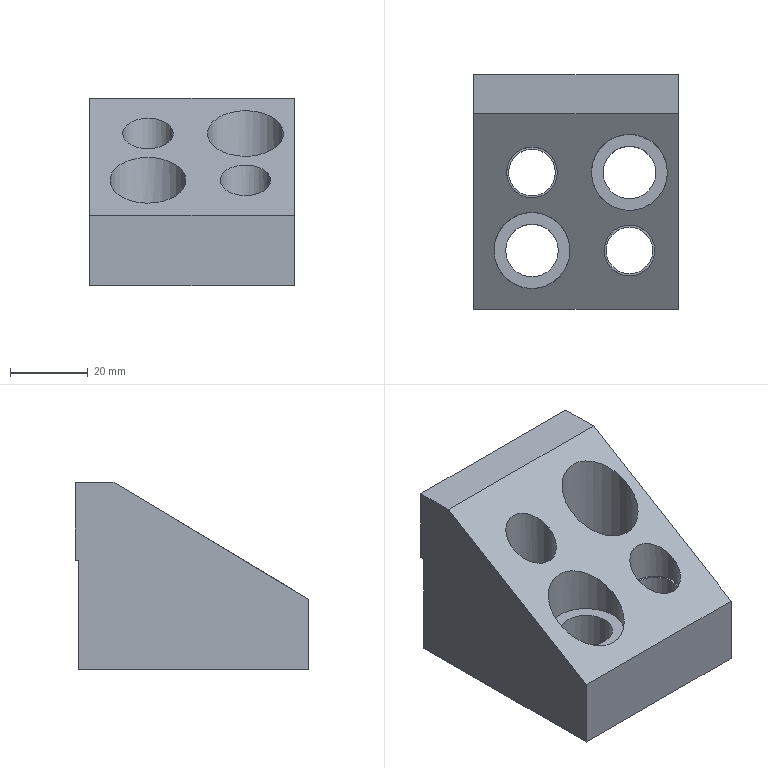Part | NX | features solid 2 | 1 solid | 21 faces | box 52.578 x 60 x 48 mm | volume 89054 mm3 | plane 13 | cylinder 8 | commonest cylinder face diameters 12 x2 13 x2 13.5 x2 19.5 x2
STEP:
#1=CARTESIAN_POINT('',(-464.,-150.,-55.));
#2=VERTEX_POINT('',#1);
#3=CARTESIAN_POINT('',(-470.,-150.,-55.));
#4=DIRECTION('',(0.,0.,1.));
#5=DIRECTION('',(1.,0.,0.));
#6=AXIS2_PLACEMENT_3D('',#3,#4,#5);
#7=CIRCLE('',#6,6.);
#8=EDGE_CURVE('',#2,#2,#7,.F.);
#9=ORIENTED_EDGE('',*,*,#8,.F.);
#10=EDGE_LOOP('',(#9));
#11=FACE_BOUND('',#10,.T.);
#12=CARTESIAN_POINT('',(-489.,-130.,-55.));
#13=VERTEX_POINT('',#12);
#14=CARTESIAN_POINT('',(-495.,-130.,-55.));
#15=DIRECTION('',(0.,0.,1.));
#16=DIRECTION('',(1.,0.,0.));
#17=AXIS2_PLACEMENT_3D('',#14,#15,#16);
#18=CIRCLE('',#17,6.);
#19=EDGE_CURVE('',#13,#13,#18,.F.);
#20=ORIENTED_EDGE('',*,*,#19,.F.);
#21=EDGE_LOOP('',(#20));
#22=FACE_BOUND('',#21,.T.);
#23=CARTESIAN_POINT('',(-488.25,-150.,-55.));
#24=VERTEX_POINT('',#23);
#25=CARTESIAN_POINT('',(-495.,-150.,-55.));
#26=DIRECTION('',(0.,0.,1.));
#27=DIRECTION('',(1.,0.,0.));
#28=AXIS2_PLACEMENT_3D('',#25,#26,#27);
#29=CIRCLE('',#28,6.75);
#30=EDGE_CURVE('',#24,#24,#29,.F.);
#31=ORIENTED_EDGE('',*,*,#30,.F.);
#32=EDGE_LOOP('',(#31));
#33=FACE_BOUND('',#32,.T.);
#34=CARTESIAN_POINT('',(-463.25,-130.,-55.));
#35=VERTEX_POINT('',#34);
#36=CARTESIAN_POINT('',(-470.,-130.,-55.));
#37=DIRECTION('',(0.,0.,1.));
#38=DIRECTION('',(1.,0.,0.));
#39=AXIS2_PLACEMENT_3D('',#36,#37,#38);
#40=CIRCLE('',#39,6.75);
#41=EDGE_CURVE('',#35,#35,#40,.F.);
#42=ORIENTED_EDGE('',*,*,#41,.F.);
#43=EDGE_LOOP('',(#42));
#44=FACE_BOUND('',#43,.T.);
#45=CARTESIAN_POINT('',(-510.,-106.,-55.));
#46=VERTEX_POINT('',#45);
#47=CARTESIAN_POINT('',(-510.,-165.,-55.));
#48=VERTEX_POINT('',#47);
#49=CARTESIAN_POINT('',(-510.,35.09,-55.));
#50=DIRECTION('',(0.,1.,0.));
#51=VECTOR('',#50,1000.);
#52=LINE('',#49,#51);
#53=EDGE_CURVE('',#46,#48,#52,.F.);
#54=ORIENTED_EDGE('',*,*,#53,.F.);
#55=CARTESIAN_POINT('',(-457.422,-106.,-55.));
#56=VERTEX_POINT('',#55);
#57=CARTESIAN_POINT('',(-457.422,-106.,-55.));
#58=DIRECTION('',(1.,0.,0.));
#59=VECTOR('',#58,1000.);
#60=LINE('',#57,#59);
#61=EDGE_CURVE('',#56,#46,#60,.F.);
#62=ORIENTED_EDGE('',*,*,#61,.F.);
#63=CARTESIAN_POINT('',(-457.422,-165.,-55.));
#64=VERTEX_POINT('',#63);
#65=CARTESIAN_POINT('',(-457.422,35.09,-55.));
#66=DIRECTION('',(0.,-1.,0.));
#67=VECTOR('',#66,1000.);
#68=LINE('',#65,#67);
#69=EDGE_CURVE('',#56,#64,#68,.T.);
#70=ORIENTED_EDGE('',*,*,#69,.T.);
#71=CARTESIAN_POINT('',(-415.478,-165.,-55.));
#72=DIRECTION('',(1.,0.,0.));
#73=VECTOR('',#72,1000.);
#74=LINE('',#71,#73);
#75=EDGE_CURVE('',#64,#48,#74,.F.);
#76=ORIENTED_EDGE('',*,*,#75,.T.);
#77=EDGE_LOOP('',(#54,#62,#70,#76));
#78=FACE_BOUND('',#77,.T.);
#79=CARTESIAN_POINT('',(-415.478,35.09,-55.));
#80=DIRECTION('',(0.,0.,1.));
#81=DIRECTION('',(1.,0.,0.));
#82=AXIS2_PLACEMENT_3D('',#79,#80,#81);
#83=PLANE('',#82);
#84=ADVANCED_FACE('',(#11,#22,#33,#44,#78),#83,.F.);
#85=CARTESIAN_POINT('',(-510.,-115.,-7.));
#86=VERTEX_POINT('',#85);
#87=CARTESIAN_POINT('',(-510.,-105.,-7.));
#88=VERTEX_POINT('',#87);
#89=CARTESIAN_POINT('',(-510.,-105.,-7.));
#90=DIRECTION('',(0.,-1.,0.));
#91=VECTOR('',#90,1000.);
#92=LINE('',#89,#91);
#93=EDGE_CURVE('',#86,#88,#92,.F.);
#94=ORIENTED_EDGE('',*,*,#93,.F.);
#95=CARTESIAN_POINT('',(-457.422,-115.,-7.));
#96=VERTEX_POINT('',#95);
#97=CARTESIAN_POINT('',(-457.422,-115.,-7.));
#98=DIRECTION('',(1.,0.,0.));
#99=VECTOR('',#98,1000.);
#100=LINE('',#97,#99);
#101=EDGE_CURVE('',#96,#86,#100,.F.);
#102=ORIENTED_EDGE('',*,*,#101,.F.);
#103=CARTESIAN_POINT('',(-457.422,-105.,-7.));
#104=VERTEX_POINT('',#103);
#105=CARTESIAN_POINT('',(-457.422,-105.,-7.));
#106=DIRECTION('',(0.,-1.,0.));
#107=VECTOR('',#106,1000.);
#108=LINE('',#105,#107);
#109=EDGE_CURVE('',#104,#96,#108,.T.);
#110=ORIENTED_EDGE('',*,*,#109,.F.);
#111=CARTESIAN_POINT('',(-457.422,-105.,-7.));
#112=DIRECTION('',(-1.,0.,0.));
#113=VECTOR('',#112,1000.);
#114=LINE('',#111,#113);
#115=EDGE_CURVE('',#104,#88,#114,.T.);
#116=ORIENTED_EDGE('',*,*,#115,.T.);
#117=EDGE_LOOP('',(#94,#102,#110,#116));
#118=FACE_BOUND('',#117,.T.);
#119=CARTESIAN_POINT('',(-457.422,-105.,-7.));
#120=DIRECTION('',(0.,0.,-1.));
#121=DIRECTION('',(-1.,0.,0.));
#122=AXIS2_PLACEMENT_3D('',#119,#120,#121);
#123=PLANE('',#122);
#124=ADVANCED_FACE('',(#118),#123,.F.);
#125=CARTESIAN_POINT('',(-457.422,-105.,-27.));
#126=VERTEX_POINT('',#125);
#127=CARTESIAN_POINT('',(-457.422,-106.,-27.));
#128=VERTEX_POINT('',#127);
#129=CARTESIAN_POINT('',(-457.422,-105.,-27.));
#130=DIRECTION('',(0.,-1.,0.));
#131=VECTOR('',#130,1000.);
#132=LINE('',#129,#131);
#133=EDGE_CURVE('',#126,#128,#132,.T.);
#134=ORIENTED_EDGE('',*,*,#133,.F.);
#135=CARTESIAN_POINT('',(-457.422,-105.,-67.));
#136=DIRECTION('',(0.,0.,1.));
#137=VECTOR('',#136,1000.);
#138=LINE('',#135,#137);
#139=EDGE_CURVE('',#126,#104,#138,.T.);
#140=ORIENTED_EDGE('',*,*,#139,.T.);
#141=ORIENTED_EDGE('',*,*,#109,.T.);
#142=CARTESIAN_POINT('',(-457.422,-165.,-37.));
#143=VERTEX_POINT('',#142);
#144=CARTESIAN_POINT('',(-457.422,-134.118,-18.471));
#145=DIRECTION('',(0.,-0.8575,-0.5145));
#146=VECTOR('',#145,1000.);
#147=LINE('',#144,#146);
#148=EDGE_CURVE('',#143,#96,#147,.F.);
#149=ORIENTED_EDGE('',*,*,#148,.F.);
#150=CARTESIAN_POINT('',(-457.422,-165.,-67.));
#151=DIRECTION('',(0.,0.,1.));
#152=VECTOR('',#151,1000.);
#153=LINE('',#150,#152);
#154=EDGE_CURVE('',#64,#143,#153,.T.);
#155=ORIENTED_EDGE('',*,*,#154,.F.);
#156=ORIENTED_EDGE('',*,*,#69,.F.);
#157=CARTESIAN_POINT('',(-457.422,-106.,-27.));
#158=DIRECTION('',(0.,0.,-1.));
#159=VECTOR('',#158,1000.);
#160=LINE('',#157,#159);
#161=EDGE_CURVE('',#128,#56,#160,.T.);
#162=ORIENTED_EDGE('',*,*,#161,.F.);
#163=EDGE_LOOP('',(#134,#140,#141,#149,#155,#156,#162));
#164=FACE_BOUND('',#163,.T.);
#165=CARTESIAN_POINT('',(-457.422,-105.,-67.));
#166=DIRECTION('',(-1.,0.,0.));
#167=DIRECTION('',(0.,0.,1.));
#168=AXIS2_PLACEMENT_3D('',#165,#166,#167);
#169=PLANE('',#168);
#170=ADVANCED_FACE('',(#164),#169,.F.);
#171=CARTESIAN_POINT('',(-510.,-165.,-37.));
#172=VERTEX_POINT('',#171);
#173=CARTESIAN_POINT('',(-510.,-165.,-67.));
#174=DIRECTION('',(0.,0.,1.));
#175=VECTOR('',#174,1000.);
#176=LINE('',#173,#175);
#177=EDGE_CURVE('',#48,#172,#176,.T.);
#178=ORIENTED_EDGE('',*,*,#177,.F.);
#179=ORIENTED_EDGE('',*,*,#75,.F.);
#180=ORIENTED_EDGE('',*,*,#154,.T.);
#181=CARTESIAN_POINT('',(-457.422,-165.,-37.));
#182=DIRECTION('',(1.,0.,0.));
#183=VECTOR('',#182,1000.);
#184=LINE('',#181,#183);
#185=EDGE_CURVE('',#172,#143,#184,.T.);
#186=ORIENTED_EDGE('',*,*,#185,.F.);
#187=EDGE_LOOP('',(#178,#179,#180,#186));
#188=FACE_BOUND('',#187,.T.);
#189=CARTESIAN_POINT('',(-457.422,-165.,-67.));
#190=DIRECTION('',(0.,-1.,0.));
#191=DIRECTION('',(0.,0.,1.));
#192=AXIS2_PLACEMENT_3D('',#189,#190,#191);
#193=PLANE('',#192);
#194=ADVANCED_FACE('',(#188),#193,.T.);
#195=CARTESIAN_POINT('',(-510.,-105.,-27.));
#196=VERTEX_POINT('',#195);
#197=CARTESIAN_POINT('',(-457.422,-105.,-27.));
#198=DIRECTION('',(1.,0.,0.));
#199=VECTOR('',#198,1000.);
#200=LINE('',#197,#199);
#201=EDGE_CURVE('',#196,#126,#200,.T.);
#202=ORIENTED_EDGE('',*,*,#201,.F.);
#203=CARTESIAN_POINT('',(-510.,-105.,-67.));
#204=DIRECTION('',(0.,0.,1.));
#205=VECTOR('',#204,1000.);
#206=LINE('',#203,#205);
#207=EDGE_CURVE('',#196,#88,#206,.T.);
#208=ORIENTED_EDGE('',*,*,#207,.T.);
#209=ORIENTED_EDGE('',*,*,#115,.F.);
#210=ORIENTED_EDGE('',*,*,#139,.F.);
#211=EDGE_LOOP('',(#202,#208,#209,#210));
#212=FACE_BOUND('',#211,.T.);
#213=CARTESIAN_POINT('',(-457.422,-105.,-67.));
#214=DIRECTION('',(0.,-1.,0.));
#215=DIRECTION('',(0.,0.,1.));
#216=AXIS2_PLACEMENT_3D('',#213,#214,#215);
#217=PLANE('',#216);
#218=ADVANCED_FACE('',(#212),#217,.F.);
#219=CARTESIAN_POINT('',(-470.,-143.5,-24.1));
#220=VERTEX_POINT('',#219);
#221=CARTESIAN_POINT('',(-470.,-150.,-28.));
#222=DIRECTION('',(0.,-0.5145,0.8575));
#223=DIRECTION('',(0.,0.8575,0.5145));
#224=AXIS2_PLACEMENT_3D('',#221,#222,#223);
#225=ELLIPSE('',#224,7.58,6.5);
#226=EDGE_CURVE('',#220,#220,#225,.T.);
#227=ORIENTED_EDGE('',*,*,#226,.F.);
#228=EDGE_LOOP('',(#227));
#229=FACE_BOUND('',#228,.T.);
#230=CARTESIAN_POINT('',(-495.,-123.5,-12.1));
#231=VERTEX_POINT('',#230);
#232=CARTESIAN_POINT('',(-495.,-130.,-16.));
#233=DIRECTION('',(0.,-0.5145,0.8575));
#234=DIRECTION('',(0.,0.8575,0.5145));
#235=AXIS2_PLACEMENT_3D('',#232,#233,#234);
#236=ELLIPSE('',#235,7.58,6.5);
#237=EDGE_CURVE('',#231,#231,#236,.T.);
#238=ORIENTED_EDGE('',*,*,#237,.F.);
#239=EDGE_LOOP('',(#238));
#240=FACE_BOUND('',#239,.T.);
#241=CARTESIAN_POINT('',(-495.,-140.25,-22.15));
#242=VERTEX_POINT('',#241);
#243=CARTESIAN_POINT('',(-495.,-150.,-28.));
#244=DIRECTION('',(0.,-0.5145,0.8575));
#245=DIRECTION('',(0.,0.8575,0.5145));
#246=AXIS2_PLACEMENT_3D('',#243,#244,#245);
#247=ELLIPSE('',#246,11.37,9.75);
#248=EDGE_CURVE('',#242,#242,#247,.T.);
#249=ORIENTED_EDGE('',*,*,#248,.F.);
#250=EDGE_LOOP('',(#249));
#251=FACE_BOUND('',#250,.T.);
#252=CARTESIAN_POINT('',(-470.,-120.25,-10.15));
#253=VERTEX_POINT('',#252);
#254=CARTESIAN_POINT('',(-470.,-130.,-16.));
#255=DIRECTION('',(0.,-0.5145,0.8575));
#256=DIRECTION('',(0.,0.8575,0.5145));
#257=AXIS2_PLACEMENT_3D('',#254,#255,#256);
#258=ELLIPSE('',#257,11.37,9.75);
#259=EDGE_CURVE('',#253,#253,#258,.T.);
#260=ORIENTED_EDGE('',*,*,#259,.F.);
#261=EDGE_LOOP('',(#260));
#262=FACE_BOUND('',#261,.T.);
#263=CARTESIAN_POINT('',(-510.,-115.,-7.));
#264=DIRECTION('',(0.,0.8575,0.5145));
#265=VECTOR('',#264,1000.);
#266=LINE('',#263,#265);
#267=EDGE_CURVE('',#172,#86,#266,.T.);
#268=ORIENTED_EDGE('',*,*,#267,.F.);
#269=ORIENTED_EDGE('',*,*,#185,.T.);
#270=ORIENTED_EDGE('',*,*,#148,.T.);
#271=ORIENTED_EDGE('',*,*,#101,.T.);
#272=EDGE_LOOP('',(#268,#269,#270,#271));
#273=FACE_BOUND('',#272,.T.);
#274=CARTESIAN_POINT('',(-478.376,-115.,-7.));
#275=DIRECTION('',(0.,-0.5145,0.8575));
#276=DIRECTION('',(0.,0.8575,0.5145));
#277=AXIS2_PLACEMENT_3D('',#274,#275,#276);
#278=PLANE('',#277);
#279=ADVANCED_FACE('',(#229,#240,#251,#262,#273),#278,.T.);
#280=CARTESIAN_POINT('',(-510.,-106.,-27.));
#281=VERTEX_POINT('',#280);
#282=CARTESIAN_POINT('',(-457.422,-106.,-27.));
#283=DIRECTION('',(1.,0.,0.));
#284=VECTOR('',#283,1000.);
#285=LINE('',#282,#284);
#286=EDGE_CURVE('',#128,#281,#285,.F.);
#287=ORIENTED_EDGE('',*,*,#286,.T.);
#288=CARTESIAN_POINT('',(-510.,-105.,-27.));
#289=DIRECTION('',(0.,1.,0.));
#290=VECTOR('',#289,1000.);
#291=LINE('',#288,#290);
#292=EDGE_CURVE('',#281,#196,#291,.T.);
#293=ORIENTED_EDGE('',*,*,#292,.T.);
#294=ORIENTED_EDGE('',*,*,#201,.T.);
#295=ORIENTED_EDGE('',*,*,#133,.T.);
#296=EDGE_LOOP('',(#287,#293,#294,#295));
#297=FACE_BOUND('',#296,.T.);
#298=CARTESIAN_POINT('',(-457.422,-105.,-27.));
#299=DIRECTION('',(0.,0.,1.));
#300=DIRECTION('',(-1.,0.,0.));
#301=AXIS2_PLACEMENT_3D('',#298,#299,#300);
#302=PLANE('',#301);
#303=ADVANCED_FACE('',(#297),#302,.F.);
#304=CARTESIAN_POINT('',(-510.,-106.,-27.));
#305=DIRECTION('',(0.,0.,-1.));
#306=VECTOR('',#305,1000.);
#307=LINE('',#304,#306);
#308=EDGE_CURVE('',#281,#46,#307,.T.);
#309=ORIENTED_EDGE('',*,*,#308,.F.);
#310=ORIENTED_EDGE('',*,*,#286,.F.);
#311=ORIENTED_EDGE('',*,*,#161,.T.);
#312=ORIENTED_EDGE('',*,*,#61,.T.);
#313=EDGE_LOOP('',(#309,#310,#311,#312));
#314=FACE_BOUND('',#313,.T.);
#315=CARTESIAN_POINT('',(-457.422,-106.,-27.));
#316=DIRECTION('',(0.,1.,0.));
#317=DIRECTION('',(0.,0.,-1.));
#318=AXIS2_PLACEMENT_3D('',#315,#316,#317);
#319=PLANE('',#318);
#320=ADVANCED_FACE('',(#314),#319,.T.);
#321=ORIENTED_EDGE('',*,*,#53,.T.);
#322=ORIENTED_EDGE('',*,*,#177,.T.);
#323=ORIENTED_EDGE('',*,*,#267,.T.);
#324=ORIENTED_EDGE('',*,*,#93,.T.);
#325=ORIENTED_EDGE('',*,*,#207,.F.);
#326=ORIENTED_EDGE('',*,*,#292,.F.);
#327=ORIENTED_EDGE('',*,*,#308,.T.);
#328=EDGE_LOOP('',(#321,#322,#323,#324,#325,#326,#327));
#329=FACE_BOUND('',#328,.T.);
#330=CARTESIAN_POINT('',(-510.,0.,-7.));
#331=DIRECTION('',(1.,0.,0.));
#332=DIRECTION('',(0.,0.,-1.));
#333=AXIS2_PLACEMENT_3D('',#330,#331,#332);
#334=PLANE('',#333);
#335=ADVANCED_FACE('',(#329),#334,.F.);
#336=ORIENTED_EDGE('',*,*,#41,.T.);
#337=EDGE_LOOP('',(#336));
#338=FACE_BOUND('',#337,.T.);
#339=CARTESIAN_POINT('',(-476.75,-130.,-35.));
#340=VERTEX_POINT('',#339);
#341=CARTESIAN_POINT('',(-470.,-130.,-35.));
#342=DIRECTION('',(0.,0.,-1.));
#343=DIRECTION('',(-1.,0.,0.));
#344=AXIS2_PLACEMENT_3D('',#341,#342,#343);
#345=CIRCLE('',#344,6.75);
#346=EDGE_CURVE('',#340,#340,#345,.F.);
#347=ORIENTED_EDGE('',*,*,#346,.T.);
#348=EDGE_LOOP('',(#347));
#349=FACE_BOUND('',#348,.T.);
#350=CARTESIAN_POINT('',(-470.,-130.,-75.));
#351=DIRECTION('',(0.,0.,1.));
#352=DIRECTION('',(1.,0.,0.));
#353=AXIS2_PLACEMENT_3D('',#350,#351,#352);
#354=CYLINDRICAL_SURFACE('',#353,6.75);
#355=ADVANCED_FACE('',(#338,#349),#354,.F.);
#356=ORIENTED_EDGE('',*,*,#346,.F.);
#357=EDGE_LOOP('',(#356));
#358=FACE_BOUND('',#357,.T.);
#359=CARTESIAN_POINT('',(-460.25,-130.,-35.));
#360=VERTEX_POINT('',#359);
#361=CARTESIAN_POINT('',(-470.,-130.,-35.));
#362=DIRECTION('',(0.,0.,1.));
#363=DIRECTION('',(1.,0.,0.));
#364=AXIS2_PLACEMENT_3D('',#361,#362,#363);
#365=CIRCLE('',#364,9.75);
#366=EDGE_CURVE('',#360,#360,#365,.T.);
#367=ORIENTED_EDGE('',*,*,#366,.T.);
#368=EDGE_LOOP('',(#367));
#369=FACE_BOUND('',#368,.T.);
#370=CARTESIAN_POINT('',(-470.,-130.,-35.));
#371=DIRECTION('',(0.,0.,-1.));
#372=DIRECTION('',(-1.,0.,0.));
#373=AXIS2_PLACEMENT_3D('',#370,#371,#372);
#374=PLANE('',#373);
#375=ADVANCED_FACE('',(#358,#369),#374,.F.);
#376=ORIENTED_EDGE('',*,*,#259,.T.);
#377=EDGE_LOOP('',(#376));
#378=FACE_BOUND('',#377,.T.);
#379=ORIENTED_EDGE('',*,*,#366,.F.);
#380=EDGE_LOOP('',(#379));
#381=FACE_BOUND('',#380,.T.);
#382=CARTESIAN_POINT('',(-470.,-130.,-35.));
#383=DIRECTION('',(0.,0.,1.));
#384=DIRECTION('',(1.,0.,0.));
#385=AXIS2_PLACEMENT_3D('',#382,#383,#384);
#386=CYLINDRICAL_SURFACE('',#385,9.75);
#387=ADVANCED_FACE('',(#378,#381),#386,.F.);
#388=ORIENTED_EDGE('',*,*,#30,.T.);
#389=EDGE_LOOP('',(#388));
#390=FACE_BOUND('',#389,.T.);
#391=CARTESIAN_POINT('',(-501.75,-150.,-35.));
#392=VERTEX_POINT('',#391);
#393=CARTESIAN_POINT('',(-495.,-150.,-35.));
#394=DIRECTION('',(0.,0.,-1.));
#395=DIRECTION('',(-1.,0.,0.));
#396=AXIS2_PLACEMENT_3D('',#393,#394,#395);
#397=CIRCLE('',#396,6.75);
#398=EDGE_CURVE('',#392,#392,#397,.F.);
#399=ORIENTED_EDGE('',*,*,#398,.T.);
#400=EDGE_LOOP('',(#399));
#401=FACE_BOUND('',#400,.T.);
#402=CARTESIAN_POINT('',(-495.,-150.,-75.));
#403=DIRECTION('',(0.,0.,1.));
#404=DIRECTION('',(1.,0.,0.));
#405=AXIS2_PLACEMENT_3D('',#402,#403,#404);
#406=CYLINDRICAL_SURFACE('',#405,6.75);
#407=ADVANCED_FACE('',(#390,#401),#406,.F.);
#408=ORIENTED_EDGE('',*,*,#398,.F.);
#409=EDGE_LOOP('',(#408));
#410=FACE_BOUND('',#409,.T.);
#411=CARTESIAN_POINT('',(-485.25,-150.,-35.));
#412=VERTEX_POINT('',#411);
#413=CARTESIAN_POINT('',(-495.,-150.,-35.));
#414=DIRECTION('',(0.,0.,1.));
#415=DIRECTION('',(1.,0.,0.));
#416=AXIS2_PLACEMENT_3D('',#413,#414,#415);
#417=CIRCLE('',#416,9.75);
#418=EDGE_CURVE('',#412,#412,#417,.T.);
#419=ORIENTED_EDGE('',*,*,#418,.T.);
#420=EDGE_LOOP('',(#419));
#421=FACE_BOUND('',#420,.T.);
#422=CARTESIAN_POINT('',(-495.,-150.,-35.));
#423=DIRECTION('',(0.,0.,-1.));
#424=DIRECTION('',(-1.,0.,0.));
#425=AXIS2_PLACEMENT_3D('',#422,#423,#424);
#426=PLANE('',#425);
#427=ADVANCED_FACE('',(#410,#421),#426,.F.);
#428=ORIENTED_EDGE('',*,*,#248,.T.);
#429=EDGE_LOOP('',(#428));
#430=FACE_BOUND('',#429,.T.);
#431=ORIENTED_EDGE('',*,*,#418,.F.);
#432=EDGE_LOOP('',(#431));
#433=FACE_BOUND('',#432,.T.);
#434=CARTESIAN_POINT('',(-495.,-150.,-35.));
#435=DIRECTION('',(0.,0.,1.));
#436=DIRECTION('',(1.,0.,0.));
#437=AXIS2_PLACEMENT_3D('',#434,#435,#436);
#438=CYLINDRICAL_SURFACE('',#437,9.75);
#439=ADVANCED_FACE('',(#430,#433),#438,.F.);
#440=ORIENTED_EDGE('',*,*,#19,.T.);
#441=EDGE_LOOP('',(#440));
#442=FACE_BOUND('',#441,.T.);
#443=CARTESIAN_POINT('',(-501.,-130.,-35.));
#444=VERTEX_POINT('',#443);
#445=CARTESIAN_POINT('',(-495.,-130.,-35.));
#446=DIRECTION('',(0.,0.,-1.));
#447=DIRECTION('',(-1.,0.,0.));
#448=AXIS2_PLACEMENT_3D('',#445,#446,#447);
#449=CIRCLE('',#448,6.);
#450=EDGE_CURVE('',#444,#444,#449,.F.);
#451=ORIENTED_EDGE('',*,*,#450,.T.);
#452=EDGE_LOOP('',(#451));
#453=FACE_BOUND('',#452,.T.);
#454=CARTESIAN_POINT('',(-495.,-130.,-75.));
#455=DIRECTION('',(0.,0.,1.));
#456=DIRECTION('',(1.,0.,0.));
#457=AXIS2_PLACEMENT_3D('',#454,#455,#456);
#458=CYLINDRICAL_SURFACE('',#457,6.);
#459=ADVANCED_FACE('',(#442,#453),#458,.F.);
#460=ORIENTED_EDGE('',*,*,#450,.F.);
#461=EDGE_LOOP('',(#460));
#462=FACE_BOUND('',#461,.T.);
#463=CARTESIAN_POINT('',(-488.5,-130.,-35.));
#464=VERTEX_POINT('',#463);
#465=CARTESIAN_POINT('',(-495.,-130.,-35.));
#466=DIRECTION('',(0.,0.,1.));
#467=DIRECTION('',(1.,0.,0.));
#468=AXIS2_PLACEMENT_3D('',#465,#466,#467);
#469=CIRCLE('',#468,6.5);
#470=EDGE_CURVE('',#464,#464,#469,.T.);
#471=ORIENTED_EDGE('',*,*,#470,.T.);
#472=EDGE_LOOP('',(#471));
#473=FACE_BOUND('',#472,.T.);
#474=CARTESIAN_POINT('',(-495.,-130.,-35.));
#475=DIRECTION('',(0.,0.,-1.));
#476=DIRECTION('',(-1.,0.,0.));
#477=AXIS2_PLACEMENT_3D('',#474,#475,#476);
#478=PLANE('',#477);
#479=ADVANCED_FACE('',(#462,#473),#478,.F.);
#480=ORIENTED_EDGE('',*,*,#237,.T.);
#481=EDGE_LOOP('',(#480));
#482=FACE_BOUND('',#481,.T.);
#483=ORIENTED_EDGE('',*,*,#470,.F.);
#484=EDGE_LOOP('',(#483));
#485=FACE_BOUND('',#484,.T.);
#486=CARTESIAN_POINT('',(-495.,-130.,-35.));
#487=DIRECTION('',(0.,0.,1.));
#488=DIRECTION('',(1.,0.,0.));
#489=AXIS2_PLACEMENT_3D('',#486,#487,#488);
#490=CYLINDRICAL_SURFACE('',#489,6.5);
#491=ADVANCED_FACE('',(#482,#485),#490,.F.);
#492=ORIENTED_EDGE('',*,*,#8,.T.);
#493=EDGE_LOOP('',(#492));
#494=FACE_BOUND('',#493,.T.);
#495=CARTESIAN_POINT('',(-476.,-150.,-35.));
#496=VERTEX_POINT('',#495);
#497=CARTESIAN_POINT('',(-470.,-150.,-35.));
#498=DIRECTION('',(0.,0.,-1.));
#499=DIRECTION('',(-1.,0.,0.));
#500=AXIS2_PLACEMENT_3D('',#497,#498,#499);
#501=CIRCLE('',#500,6.);
#502=EDGE_CURVE('',#496,#496,#501,.F.);
#503=ORIENTED_EDGE('',*,*,#502,.T.);
#504=EDGE_LOOP('',(#503));
#505=FACE_BOUND('',#504,.T.);
#506=CARTESIAN_POINT('',(-470.,-150.,-75.));
#507=DIRECTION('',(0.,0.,1.));
#508=DIRECTION('',(1.,0.,0.));
#509=AXIS2_PLACEMENT_3D('',#506,#507,#508);
#510=CYLINDRICAL_SURFACE('',#509,6.);
#511=ADVANCED_FACE('',(#494,#505),#510,.F.);
#512=ORIENTED_EDGE('',*,*,#502,.F.);
#513=EDGE_LOOP('',(#512));
#514=FACE_BOUND('',#513,.T.);
#515=CARTESIAN_POINT('',(-463.5,-150.,-35.));
#516=VERTEX_POINT('',#515);
#517=CARTESIAN_POINT('',(-470.,-150.,-35.));
#518=DIRECTION('',(0.,0.,1.));
#519=DIRECTION('',(1.,0.,0.));
#520=AXIS2_PLACEMENT_3D('',#517,#518,#519);
#521=CIRCLE('',#520,6.5);
#522=EDGE_CURVE('',#516,#516,#521,.T.);
#523=ORIENTED_EDGE('',*,*,#522,.T.);
#524=EDGE_LOOP('',(#523));
#525=FACE_BOUND('',#524,.T.);
#526=CARTESIAN_POINT('',(-470.,-150.,-35.));
#527=DIRECTION('',(0.,0.,-1.));
#528=DIRECTION('',(-1.,0.,0.));
#529=AXIS2_PLACEMENT_3D('',#526,#527,#528);
#530=PLANE('',#529);
#531=ADVANCED_FACE('',(#514,#525),#530,.F.);
#532=ORIENTED_EDGE('',*,*,#226,.T.);
#533=EDGE_LOOP('',(#532));
#534=FACE_BOUND('',#533,.T.);
#535=ORIENTED_EDGE('',*,*,#522,.F.);
#536=EDGE_LOOP('',(#535));
#537=FACE_BOUND('',#536,.T.);
#538=CARTESIAN_POINT('',(-470.,-150.,-35.));
#539=DIRECTION('',(0.,0.,1.));
#540=DIRECTION('',(1.,0.,0.));
#541=AXIS2_PLACEMENT_3D('',#538,#539,#540);
#542=CYLINDRICAL_SURFACE('',#541,6.5);
#543=ADVANCED_FACE('',(#534,#537),#542,.F.);
#544=CLOSED_SHELL('',(#84,#124,#170,#194,#218,#279,#303,#320,#335,#355,#375,#387,#407,#427,#439,#459,#479,#491,#511,#531,#543));
#545=MANIFOLD_SOLID_BREP('',#544);
#546=(LENGTH_UNIT()NAMED_UNIT(*)SI_UNIT(.MILLI.,.METRE.));
#547=UNCERTAINTY_MEASURE_WITH_UNIT(LENGTH_MEASURE(0.00001),#546,'','');
#548=(NAMED_UNIT(*)PLANE_ANGLE_UNIT()SI_UNIT($,.RADIAN.));
#549=(NAMED_UNIT(*)SI_UNIT($,.STERADIAN.)SOLID_ANGLE_UNIT());
#550=(GEOMETRIC_REPRESENTATION_CONTEXT(3)GLOBAL_UNCERTAINTY_ASSIGNED_CONTEXT((#547))GLOBAL_UNIT_ASSIGNED_CONTEXT((#546,#548,#549))REPRESENTATION_CONTEXT('',''));
#551=ADVANCED_BREP_SHAPE_REPRESENTATION('',(#545),#550);